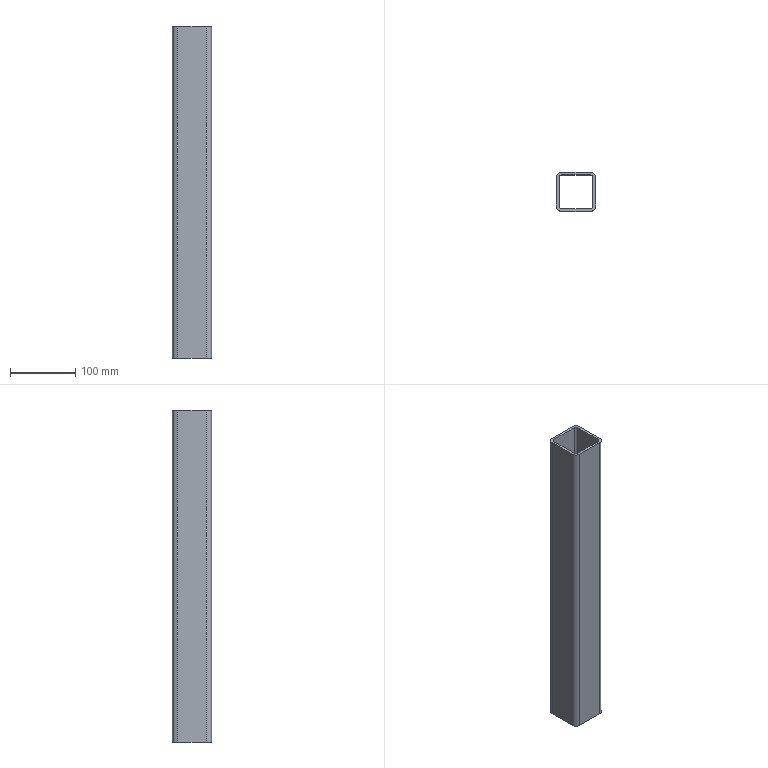Part | SolidWorks | features ICE 1, LibraryFeature 1 | 1 solid | 18 faces | box 60 x 60 x 510 mm | volume 435946 mm3 | plane 10 | cylinder 8 | commonest cylinder face diameters 8 x4 16 x4
STEP:
#1=CARTESIAN_POINT('',(22.,30.,0.));
#2=VERTEX_POINT('',#1);
#3=CARTESIAN_POINT('',(-22.,30.,0.));
#4=VERTEX_POINT('',#3);
#5=CARTESIAN_POINT('',(0.,30.,0.));
#6=DIRECTION('',(-1.,0.,0.));
#7=VECTOR('',#6,1000.);
#8=LINE('',#5,#7);
#9=EDGE_CURVE('',#2,#4,#8,.T.);
#10=ORIENTED_EDGE('',*,*,#9,.T.);
#11=CARTESIAN_POINT('',(-22.,30.,510.));
#12=VERTEX_POINT('',#11);
#13=CARTESIAN_POINT('',(-22.,30.,510.));
#14=DIRECTION('',(0.,0.,-1.));
#15=VECTOR('',#14,1000.);
#16=LINE('',#13,#15);
#17=EDGE_CURVE('',#12,#4,#16,.T.);
#18=ORIENTED_EDGE('',*,*,#17,.F.);
#19=CARTESIAN_POINT('',(22.,30.,510.));
#20=VERTEX_POINT('',#19);
#21=CARTESIAN_POINT('',(0.,30.,510.));
#22=DIRECTION('',(-1.,0.,0.));
#23=VECTOR('',#22,1000.);
#24=LINE('',#21,#23);
#25=EDGE_CURVE('',#20,#12,#24,.T.);
#26=ORIENTED_EDGE('',*,*,#25,.F.);
#27=CARTESIAN_POINT('',(22.,30.,510.));
#28=DIRECTION('',(0.,0.,-1.));
#29=VECTOR('',#28,1000.);
#30=LINE('',#27,#29);
#31=EDGE_CURVE('',#20,#2,#30,.T.);
#32=ORIENTED_EDGE('',*,*,#31,.T.);
#33=EDGE_LOOP('',(#10,#18,#26,#32));
#34=FACE_OUTER_BOUND('',#33,.T.);
#35=CARTESIAN_POINT('',(0.,30.,510.));
#36=DIRECTION('',(0.,-1.,0.));
#37=DIRECTION('',(0.,0.,-1.));
#38=AXIS2_PLACEMENT_3D('',#35,#36,#37);
#39=PLANE('',#38);
#40=ADVANCED_FACE('',(#34),#39,.F.);
#41=CARTESIAN_POINT('',(-30.,22.,0.));
#42=VERTEX_POINT('',#41);
#43=CARTESIAN_POINT('',(-22.,22.,0.));
#44=DIRECTION('',(0.,0.,1.));
#45=DIRECTION('',(1.,0.,0.));
#46=AXIS2_PLACEMENT_3D('',#43,#44,#45);
#47=CIRCLE('',#46,8.);
#48=EDGE_CURVE('',#4,#42,#47,.T.);
#49=ORIENTED_EDGE('',*,*,#48,.T.);
#50=CARTESIAN_POINT('',(-30.,22.,510.));
#51=VERTEX_POINT('',#50);
#52=CARTESIAN_POINT('',(-30.,22.,510.));
#53=DIRECTION('',(0.,0.,-1.));
#54=VECTOR('',#53,1000.);
#55=LINE('',#52,#54);
#56=EDGE_CURVE('',#51,#42,#55,.T.);
#57=ORIENTED_EDGE('',*,*,#56,.F.);
#58=CARTESIAN_POINT('',(-22.,22.,510.));
#59=DIRECTION('',(0.,0.,1.));
#60=DIRECTION('',(1.,0.,0.));
#61=AXIS2_PLACEMENT_3D('',#58,#59,#60);
#62=CIRCLE('',#61,8.);
#63=EDGE_CURVE('',#12,#51,#62,.T.);
#64=ORIENTED_EDGE('',*,*,#63,.F.);
#65=ORIENTED_EDGE('',*,*,#17,.T.);
#66=EDGE_LOOP('',(#49,#57,#64,#65));
#67=FACE_OUTER_BOUND('',#66,.T.);
#68=CARTESIAN_POINT('',(-22.,22.,510.));
#69=DIRECTION('',(0.,0.,-1.));
#70=DIRECTION('',(-1.,0.,0.));
#71=AXIS2_PLACEMENT_3D('',#68,#69,#70);
#72=CYLINDRICAL_SURFACE('',#71,8.);
#73=ADVANCED_FACE('',(#67),#72,.T.);
#74=CARTESIAN_POINT('',(-30.,-22.,0.));
#75=VERTEX_POINT('',#74);
#76=CARTESIAN_POINT('',(-30.,0.,0.));
#77=DIRECTION('',(0.,1.,0.));
#78=VECTOR('',#77,1000.);
#79=LINE('',#76,#78);
#80=EDGE_CURVE('',#75,#42,#79,.T.);
#81=ORIENTED_EDGE('',*,*,#80,.F.);
#82=CARTESIAN_POINT('',(-30.,-22.,510.));
#83=VERTEX_POINT('',#82);
#84=CARTESIAN_POINT('',(-30.,-22.,510.));
#85=DIRECTION('',(0.,0.,-1.));
#86=VECTOR('',#85,1000.);
#87=LINE('',#84,#86);
#88=EDGE_CURVE('',#83,#75,#87,.T.);
#89=ORIENTED_EDGE('',*,*,#88,.F.);
#90=CARTESIAN_POINT('',(-30.,0.,510.));
#91=DIRECTION('',(0.,1.,0.));
#92=VECTOR('',#91,1000.);
#93=LINE('',#90,#92);
#94=EDGE_CURVE('',#83,#51,#93,.T.);
#95=ORIENTED_EDGE('',*,*,#94,.T.);
#96=ORIENTED_EDGE('',*,*,#56,.T.);
#97=EDGE_LOOP('',(#81,#89,#95,#96));
#98=FACE_OUTER_BOUND('',#97,.T.);
#99=CARTESIAN_POINT('',(-30.,0.,510.));
#100=DIRECTION('',(-1.,0.,0.));
#101=DIRECTION('',(0.,0.,1.));
#102=AXIS2_PLACEMENT_3D('',#99,#100,#101);
#103=PLANE('',#102);
#104=ADVANCED_FACE('',(#98),#103,.T.);
#105=CARTESIAN_POINT('',(-22.,-30.,0.));
#106=VERTEX_POINT('',#105);
#107=CARTESIAN_POINT('',(-22.,-22.,0.));
#108=DIRECTION('',(0.,0.,1.));
#109=DIRECTION('',(1.,0.,0.));
#110=AXIS2_PLACEMENT_3D('',#107,#108,#109);
#111=CIRCLE('',#110,8.);
#112=EDGE_CURVE('',#75,#106,#111,.T.);
#113=ORIENTED_EDGE('',*,*,#112,.T.);
#114=CARTESIAN_POINT('',(-22.,-30.,510.));
#115=VERTEX_POINT('',#114);
#116=CARTESIAN_POINT('',(-22.,-30.,510.));
#117=DIRECTION('',(0.,0.,-1.));
#118=VECTOR('',#117,1000.);
#119=LINE('',#116,#118);
#120=EDGE_CURVE('',#115,#106,#119,.T.);
#121=ORIENTED_EDGE('',*,*,#120,.F.);
#122=CARTESIAN_POINT('',(-22.,-22.,510.));
#123=DIRECTION('',(0.,0.,1.));
#124=DIRECTION('',(1.,0.,0.));
#125=AXIS2_PLACEMENT_3D('',#122,#123,#124);
#126=CIRCLE('',#125,8.);
#127=EDGE_CURVE('',#83,#115,#126,.T.);
#128=ORIENTED_EDGE('',*,*,#127,.F.);
#129=ORIENTED_EDGE('',*,*,#88,.T.);
#130=EDGE_LOOP('',(#113,#121,#128,#129));
#131=FACE_OUTER_BOUND('',#130,.T.);
#132=CARTESIAN_POINT('',(-22.,-22.,510.));
#133=DIRECTION('',(0.,0.,-1.));
#134=DIRECTION('',(-1.,0.,0.));
#135=AXIS2_PLACEMENT_3D('',#132,#133,#134);
#136=CYLINDRICAL_SURFACE('',#135,8.);
#137=ADVANCED_FACE('',(#131),#136,.T.);
#138=CARTESIAN_POINT('',(22.,-30.,0.));
#139=VERTEX_POINT('',#138);
#140=CARTESIAN_POINT('',(0.,-30.,0.));
#141=DIRECTION('',(1.,0.,0.));
#142=VECTOR('',#141,1000.);
#143=LINE('',#140,#142);
#144=EDGE_CURVE('',#106,#139,#143,.T.);
#145=ORIENTED_EDGE('',*,*,#144,.T.);
#146=CARTESIAN_POINT('',(22.,-30.,510.));
#147=VERTEX_POINT('',#146);
#148=CARTESIAN_POINT('',(22.,-30.,510.));
#149=DIRECTION('',(0.,0.,-1.));
#150=VECTOR('',#149,1000.);
#151=LINE('',#148,#150);
#152=EDGE_CURVE('',#147,#139,#151,.T.);
#153=ORIENTED_EDGE('',*,*,#152,.F.);
#154=CARTESIAN_POINT('',(0.,-30.,510.));
#155=DIRECTION('',(1.,0.,0.));
#156=VECTOR('',#155,1000.);
#157=LINE('',#154,#156);
#158=EDGE_CURVE('',#115,#147,#157,.T.);
#159=ORIENTED_EDGE('',*,*,#158,.F.);
#160=ORIENTED_EDGE('',*,*,#120,.T.);
#161=EDGE_LOOP('',(#145,#153,#159,#160));
#162=FACE_OUTER_BOUND('',#161,.T.);
#163=CARTESIAN_POINT('',(0.,-30.,510.));
#164=DIRECTION('',(0.,1.,0.));
#165=DIRECTION('',(0.,0.,1.));
#166=AXIS2_PLACEMENT_3D('',#163,#164,#165);
#167=PLANE('',#166);
#168=ADVANCED_FACE('',(#162),#167,.F.);
#169=CARTESIAN_POINT('',(30.,-22.,0.));
#170=VERTEX_POINT('',#169);
#171=CARTESIAN_POINT('',(22.,-22.,0.));
#172=DIRECTION('',(0.,0.,1.));
#173=DIRECTION('',(1.,0.,0.));
#174=AXIS2_PLACEMENT_3D('',#171,#172,#173);
#175=CIRCLE('',#174,8.);
#176=EDGE_CURVE('',#139,#170,#175,.T.);
#177=ORIENTED_EDGE('',*,*,#176,.T.);
#178=CARTESIAN_POINT('',(30.,-22.,510.));
#179=VERTEX_POINT('',#178);
#180=CARTESIAN_POINT('',(30.,-22.,510.));
#181=DIRECTION('',(0.,0.,-1.));
#182=VECTOR('',#181,1000.);
#183=LINE('',#180,#182);
#184=EDGE_CURVE('',#179,#170,#183,.T.);
#185=ORIENTED_EDGE('',*,*,#184,.F.);
#186=CARTESIAN_POINT('',(22.,-22.,510.));
#187=DIRECTION('',(0.,0.,1.));
#188=DIRECTION('',(1.,0.,0.));
#189=AXIS2_PLACEMENT_3D('',#186,#187,#188);
#190=CIRCLE('',#189,8.);
#191=EDGE_CURVE('',#147,#179,#190,.T.);
#192=ORIENTED_EDGE('',*,*,#191,.F.);
#193=ORIENTED_EDGE('',*,*,#152,.T.);
#194=EDGE_LOOP('',(#177,#185,#192,#193));
#195=FACE_OUTER_BOUND('',#194,.T.);
#196=CARTESIAN_POINT('',(22.,-22.,510.));
#197=DIRECTION('',(0.,0.,-1.));
#198=DIRECTION('',(-1.,0.,0.));
#199=AXIS2_PLACEMENT_3D('',#196,#197,#198);
#200=CYLINDRICAL_SURFACE('',#199,8.);
#201=ADVANCED_FACE('',(#195),#200,.T.);
#202=CARTESIAN_POINT('',(30.,22.,0.));
#203=VERTEX_POINT('',#202);
#204=CARTESIAN_POINT('',(30.,0.,0.));
#205=DIRECTION('',(0.,-1.,0.));
#206=VECTOR('',#205,1000.);
#207=LINE('',#204,#206);
#208=EDGE_CURVE('',#203,#170,#207,.T.);
#209=ORIENTED_EDGE('',*,*,#208,.F.);
#210=CARTESIAN_POINT('',(30.,22.,510.));
#211=VERTEX_POINT('',#210);
#212=CARTESIAN_POINT('',(30.,22.,510.));
#213=DIRECTION('',(0.,0.,-1.));
#214=VECTOR('',#213,1000.);
#215=LINE('',#212,#214);
#216=EDGE_CURVE('',#211,#203,#215,.T.);
#217=ORIENTED_EDGE('',*,*,#216,.F.);
#218=CARTESIAN_POINT('',(30.,0.,510.));
#219=DIRECTION('',(0.,-1.,0.));
#220=VECTOR('',#219,1000.);
#221=LINE('',#218,#220);
#222=EDGE_CURVE('',#211,#179,#221,.T.);
#223=ORIENTED_EDGE('',*,*,#222,.T.);
#224=ORIENTED_EDGE('',*,*,#184,.T.);
#225=EDGE_LOOP('',(#209,#217,#223,#224));
#226=FACE_OUTER_BOUND('',#225,.T.);
#227=CARTESIAN_POINT('',(30.,0.,510.));
#228=DIRECTION('',(1.,0.,0.));
#229=DIRECTION('',(0.,0.,-1.));
#230=AXIS2_PLACEMENT_3D('',#227,#228,#229);
#231=PLANE('',#230);
#232=ADVANCED_FACE('',(#226),#231,.T.);
#233=CARTESIAN_POINT('',(-26.,-22.,0.));
#234=VERTEX_POINT('',#233);
#235=CARTESIAN_POINT('',(-22.,-26.,0.));
#236=VERTEX_POINT('',#235);
#237=CARTESIAN_POINT('',(-22.,-22.,0.));
#238=DIRECTION('',(0.,0.,1.));
#239=DIRECTION('',(1.,0.,0.));
#240=AXIS2_PLACEMENT_3D('',#237,#238,#239);
#241=CIRCLE('',#240,4.);
#242=EDGE_CURVE('',#234,#236,#241,.T.);
#243=ORIENTED_EDGE('',*,*,#242,.F.);
#244=CARTESIAN_POINT('',(-26.,-22.,510.));
#245=VERTEX_POINT('',#244);
#246=CARTESIAN_POINT('',(-26.,-22.,510.));
#247=DIRECTION('',(0.,0.,-1.));
#248=VECTOR('',#247,1000.);
#249=LINE('',#246,#248);
#250=EDGE_CURVE('',#245,#234,#249,.T.);
#251=ORIENTED_EDGE('',*,*,#250,.F.);
#252=CARTESIAN_POINT('',(-22.,-26.,510.));
#253=VERTEX_POINT('',#252);
#254=CARTESIAN_POINT('',(-22.,-22.,510.));
#255=DIRECTION('',(0.,0.,1.));
#256=DIRECTION('',(1.,0.,0.));
#257=AXIS2_PLACEMENT_3D('',#254,#255,#256);
#258=CIRCLE('',#257,4.);
#259=EDGE_CURVE('',#245,#253,#258,.T.);
#260=ORIENTED_EDGE('',*,*,#259,.T.);
#261=CARTESIAN_POINT('',(-22.,-26.,510.));
#262=DIRECTION('',(0.,0.,-1.));
#263=VECTOR('',#262,1000.);
#264=LINE('',#261,#263);
#265=EDGE_CURVE('',#253,#236,#264,.T.);
#266=ORIENTED_EDGE('',*,*,#265,.T.);
#267=EDGE_LOOP('',(#243,#251,#260,#266));
#268=FACE_OUTER_BOUND('',#267,.T.);
#269=CARTESIAN_POINT('',(-22.,-22.,510.));
#270=DIRECTION('',(0.,0.,-1.));
#271=DIRECTION('',(-1.,0.,0.));
#272=AXIS2_PLACEMENT_3D('',#269,#270,#271);
#273=CYLINDRICAL_SURFACE('',#272,4.);
#274=ADVANCED_FACE('',(#268),#273,.F.);
#275=CARTESIAN_POINT('',(-26.,22.,0.));
#276=VERTEX_POINT('',#275);
#277=CARTESIAN_POINT('',(-26.,0.,0.));
#278=DIRECTION('',(0.,1.,0.));
#279=VECTOR('',#278,1000.);
#280=LINE('',#277,#279);
#281=EDGE_CURVE('',#234,#276,#280,.T.);
#282=ORIENTED_EDGE('',*,*,#281,.T.);
#283=CARTESIAN_POINT('',(-26.,22.,510.));
#284=VERTEX_POINT('',#283);
#285=CARTESIAN_POINT('',(-26.,22.,510.));
#286=DIRECTION('',(0.,0.,-1.));
#287=VECTOR('',#286,1000.);
#288=LINE('',#285,#287);
#289=EDGE_CURVE('',#284,#276,#288,.T.);
#290=ORIENTED_EDGE('',*,*,#289,.F.);
#291=CARTESIAN_POINT('',(-26.,0.,510.));
#292=DIRECTION('',(0.,1.,0.));
#293=VECTOR('',#292,1000.);
#294=LINE('',#291,#293);
#295=EDGE_CURVE('',#245,#284,#294,.T.);
#296=ORIENTED_EDGE('',*,*,#295,.F.);
#297=ORIENTED_EDGE('',*,*,#250,.T.);
#298=EDGE_LOOP('',(#282,#290,#296,#297));
#299=FACE_OUTER_BOUND('',#298,.T.);
#300=CARTESIAN_POINT('',(-26.,0.,510.));
#301=DIRECTION('',(-1.,0.,0.));
#302=DIRECTION('',(0.,0.,1.));
#303=AXIS2_PLACEMENT_3D('',#300,#301,#302);
#304=PLANE('',#303);
#305=ADVANCED_FACE('',(#299),#304,.F.);
#306=CARTESIAN_POINT('',(-22.,26.,0.));
#307=VERTEX_POINT('',#306);
#308=CARTESIAN_POINT('',(-22.,22.,0.));
#309=DIRECTION('',(0.,0.,1.));
#310=DIRECTION('',(1.,0.,0.));
#311=AXIS2_PLACEMENT_3D('',#308,#309,#310);
#312=CIRCLE('',#311,4.);
#313=EDGE_CURVE('',#307,#276,#312,.T.);
#314=ORIENTED_EDGE('',*,*,#313,.F.);
#315=CARTESIAN_POINT('',(-22.,26.,510.));
#316=VERTEX_POINT('',#315);
#317=CARTESIAN_POINT('',(-22.,26.,510.));
#318=DIRECTION('',(0.,0.,-1.));
#319=VECTOR('',#318,1000.);
#320=LINE('',#317,#319);
#321=EDGE_CURVE('',#316,#307,#320,.T.);
#322=ORIENTED_EDGE('',*,*,#321,.F.);
#323=CARTESIAN_POINT('',(-22.,22.,510.));
#324=DIRECTION('',(0.,0.,1.));
#325=DIRECTION('',(1.,0.,0.));
#326=AXIS2_PLACEMENT_3D('',#323,#324,#325);
#327=CIRCLE('',#326,4.);
#328=EDGE_CURVE('',#316,#284,#327,.T.);
#329=ORIENTED_EDGE('',*,*,#328,.T.);
#330=ORIENTED_EDGE('',*,*,#289,.T.);
#331=EDGE_LOOP('',(#314,#322,#329,#330));
#332=FACE_OUTER_BOUND('',#331,.T.);
#333=CARTESIAN_POINT('',(-22.,22.,510.));
#334=DIRECTION('',(0.,0.,-1.));
#335=DIRECTION('',(-1.,0.,0.));
#336=AXIS2_PLACEMENT_3D('',#333,#334,#335);
#337=CYLINDRICAL_SURFACE('',#336,4.);
#338=ADVANCED_FACE('',(#332),#337,.F.);
#339=CARTESIAN_POINT('',(22.,26.,0.));
#340=VERTEX_POINT('',#339);
#341=CARTESIAN_POINT('',(0.,26.,0.));
#342=DIRECTION('',(-1.,0.,0.));
#343=VECTOR('',#342,1000.);
#344=LINE('',#341,#343);
#345=EDGE_CURVE('',#340,#307,#344,.T.);
#346=ORIENTED_EDGE('',*,*,#345,.F.);
#347=CARTESIAN_POINT('',(22.,26.,510.));
#348=VERTEX_POINT('',#347);
#349=CARTESIAN_POINT('',(22.,26.,510.));
#350=DIRECTION('',(0.,0.,-1.));
#351=VECTOR('',#350,1000.);
#352=LINE('',#349,#351);
#353=EDGE_CURVE('',#348,#340,#352,.T.);
#354=ORIENTED_EDGE('',*,*,#353,.F.);
#355=CARTESIAN_POINT('',(0.,26.,510.));
#356=DIRECTION('',(-1.,0.,0.));
#357=VECTOR('',#356,1000.);
#358=LINE('',#355,#357);
#359=EDGE_CURVE('',#348,#316,#358,.T.);
#360=ORIENTED_EDGE('',*,*,#359,.T.);
#361=ORIENTED_EDGE('',*,*,#321,.T.);
#362=EDGE_LOOP('',(#346,#354,#360,#361));
#363=FACE_OUTER_BOUND('',#362,.T.);
#364=CARTESIAN_POINT('',(0.,26.,510.));
#365=DIRECTION('',(0.,-1.,0.));
#366=DIRECTION('',(0.,0.,-1.));
#367=AXIS2_PLACEMENT_3D('',#364,#365,#366);
#368=PLANE('',#367);
#369=ADVANCED_FACE('',(#363),#368,.T.);
#370=CARTESIAN_POINT('',(26.,22.,0.));
#371=VERTEX_POINT('',#370);
#372=CARTESIAN_POINT('',(22.,22.,0.));
#373=DIRECTION('',(0.,0.,1.));
#374=DIRECTION('',(1.,0.,0.));
#375=AXIS2_PLACEMENT_3D('',#372,#373,#374);
#376=CIRCLE('',#375,4.);
#377=EDGE_CURVE('',#371,#340,#376,.T.);
#378=ORIENTED_EDGE('',*,*,#377,.F.);
#379=CARTESIAN_POINT('',(26.,22.,510.));
#380=VERTEX_POINT('',#379);
#381=CARTESIAN_POINT('',(26.,22.,510.));
#382=DIRECTION('',(0.,0.,-1.));
#383=VECTOR('',#382,1000.);
#384=LINE('',#381,#383);
#385=EDGE_CURVE('',#380,#371,#384,.T.);
#386=ORIENTED_EDGE('',*,*,#385,.F.);
#387=CARTESIAN_POINT('',(22.,22.,510.));
#388=DIRECTION('',(0.,0.,1.));
#389=DIRECTION('',(1.,0.,0.));
#390=AXIS2_PLACEMENT_3D('',#387,#388,#389);
#391=CIRCLE('',#390,4.);
#392=EDGE_CURVE('',#380,#348,#391,.T.);
#393=ORIENTED_EDGE('',*,*,#392,.T.);
#394=ORIENTED_EDGE('',*,*,#353,.T.);
#395=EDGE_LOOP('',(#378,#386,#393,#394));
#396=FACE_OUTER_BOUND('',#395,.T.);
#397=CARTESIAN_POINT('',(22.,22.,510.));
#398=DIRECTION('',(0.,0.,-1.));
#399=DIRECTION('',(-1.,0.,0.));
#400=AXIS2_PLACEMENT_3D('',#397,#398,#399);
#401=CYLINDRICAL_SURFACE('',#400,4.);
#402=ADVANCED_FACE('',(#396),#401,.F.);
#403=CARTESIAN_POINT('',(26.,-22.,0.));
#404=VERTEX_POINT('',#403);
#405=CARTESIAN_POINT('',(26.,0.,0.));
#406=DIRECTION('',(0.,-1.,0.));
#407=VECTOR('',#406,1000.);
#408=LINE('',#405,#407);
#409=EDGE_CURVE('',#371,#404,#408,.T.);
#410=ORIENTED_EDGE('',*,*,#409,.T.);
#411=CARTESIAN_POINT('',(26.,-22.,510.));
#412=VERTEX_POINT('',#411);
#413=CARTESIAN_POINT('',(26.,-22.,510.));
#414=DIRECTION('',(0.,0.,-1.));
#415=VECTOR('',#414,1000.);
#416=LINE('',#413,#415);
#417=EDGE_CURVE('',#412,#404,#416,.T.);
#418=ORIENTED_EDGE('',*,*,#417,.F.);
#419=CARTESIAN_POINT('',(26.,0.,510.));
#420=DIRECTION('',(0.,-1.,0.));
#421=VECTOR('',#420,1000.);
#422=LINE('',#419,#421);
#423=EDGE_CURVE('',#380,#412,#422,.T.);
#424=ORIENTED_EDGE('',*,*,#423,.F.);
#425=ORIENTED_EDGE('',*,*,#385,.T.);
#426=EDGE_LOOP('',(#410,#418,#424,#425));
#427=FACE_OUTER_BOUND('',#426,.T.);
#428=CARTESIAN_POINT('',(26.,0.,510.));
#429=DIRECTION('',(1.,0.,0.));
#430=DIRECTION('',(0.,0.,-1.));
#431=AXIS2_PLACEMENT_3D('',#428,#429,#430);
#432=PLANE('',#431);
#433=ADVANCED_FACE('',(#427),#432,.F.);
#434=CARTESIAN_POINT('',(22.,-26.,0.));
#435=VERTEX_POINT('',#434);
#436=CARTESIAN_POINT('',(22.,-22.,0.));
#437=DIRECTION('',(0.,0.,1.));
#438=DIRECTION('',(1.,0.,0.));
#439=AXIS2_PLACEMENT_3D('',#436,#437,#438);
#440=CIRCLE('',#439,4.);
#441=EDGE_CURVE('',#435,#404,#440,.T.);
#442=ORIENTED_EDGE('',*,*,#441,.F.);
#443=CARTESIAN_POINT('',(22.,-26.,510.));
#444=VERTEX_POINT('',#443);
#445=CARTESIAN_POINT('',(22.,-26.,510.));
#446=DIRECTION('',(0.,0.,-1.));
#447=VECTOR('',#446,1000.);
#448=LINE('',#445,#447);
#449=EDGE_CURVE('',#444,#435,#448,.T.);
#450=ORIENTED_EDGE('',*,*,#449,.F.);
#451=CARTESIAN_POINT('',(22.,-22.,510.));
#452=DIRECTION('',(0.,0.,1.));
#453=DIRECTION('',(1.,0.,0.));
#454=AXIS2_PLACEMENT_3D('',#451,#452,#453);
#455=CIRCLE('',#454,4.);
#456=EDGE_CURVE('',#444,#412,#455,.T.);
#457=ORIENTED_EDGE('',*,*,#456,.T.);
#458=ORIENTED_EDGE('',*,*,#417,.T.);
#459=EDGE_LOOP('',(#442,#450,#457,#458));
#460=FACE_OUTER_BOUND('',#459,.T.);
#461=CARTESIAN_POINT('',(22.,-22.,510.));
#462=DIRECTION('',(0.,0.,-1.));
#463=DIRECTION('',(-1.,0.,0.));
#464=AXIS2_PLACEMENT_3D('',#461,#462,#463);
#465=CYLINDRICAL_SURFACE('',#464,4.);
#466=ADVANCED_FACE('',(#460),#465,.F.);
#467=CARTESIAN_POINT('',(0.,-26.,0.));
#468=DIRECTION('',(1.,0.,0.));
#469=VECTOR('',#468,1000.);
#470=LINE('',#467,#469);
#471=EDGE_CURVE('',#236,#435,#470,.T.);
#472=ORIENTED_EDGE('',*,*,#471,.F.);
#473=ORIENTED_EDGE('',*,*,#265,.F.);
#474=CARTESIAN_POINT('',(0.,-26.,510.));
#475=DIRECTION('',(1.,0.,0.));
#476=VECTOR('',#475,1000.);
#477=LINE('',#474,#476);
#478=EDGE_CURVE('',#253,#444,#477,.T.);
#479=ORIENTED_EDGE('',*,*,#478,.T.);
#480=ORIENTED_EDGE('',*,*,#449,.T.);
#481=EDGE_LOOP('',(#472,#473,#479,#480));
#482=FACE_OUTER_BOUND('',#481,.T.);
#483=CARTESIAN_POINT('',(0.,-26.,510.));
#484=DIRECTION('',(0.,1.,0.));
#485=DIRECTION('',(0.,0.,1.));
#486=AXIS2_PLACEMENT_3D('',#483,#484,#485);
#487=PLANE('',#486);
#488=ADVANCED_FACE('',(#482),#487,.T.);
#489=CARTESIAN_POINT('',(22.,22.,0.));
#490=DIRECTION('',(0.,0.,1.));
#491=DIRECTION('',(1.,0.,0.));
#492=AXIS2_PLACEMENT_3D('',#489,#490,#491);
#493=CIRCLE('',#492,8.);
#494=EDGE_CURVE('',#203,#2,#493,.T.);
#495=ORIENTED_EDGE('',*,*,#494,.T.);
#496=ORIENTED_EDGE('',*,*,#31,.F.);
#497=CARTESIAN_POINT('',(22.,22.,510.));
#498=DIRECTION('',(0.,0.,1.));
#499=DIRECTION('',(1.,0.,0.));
#500=AXIS2_PLACEMENT_3D('',#497,#498,#499);
#501=CIRCLE('',#500,8.);
#502=EDGE_CURVE('',#211,#20,#501,.T.);
#503=ORIENTED_EDGE('',*,*,#502,.F.);
#504=ORIENTED_EDGE('',*,*,#216,.T.);
#505=EDGE_LOOP('',(#495,#496,#503,#504));
#506=FACE_OUTER_BOUND('',#505,.T.);
#507=CARTESIAN_POINT('',(22.,22.,510.));
#508=DIRECTION('',(0.,0.,-1.));
#509=DIRECTION('',(-1.,0.,0.));
#510=AXIS2_PLACEMENT_3D('',#507,#508,#509);
#511=CYLINDRICAL_SURFACE('',#510,8.);
#512=ADVANCED_FACE('',(#506),#511,.T.);
#513=ORIENTED_EDGE('',*,*,#259,.F.);
#514=ORIENTED_EDGE('',*,*,#295,.T.);
#515=ORIENTED_EDGE('',*,*,#328,.F.);
#516=ORIENTED_EDGE('',*,*,#359,.F.);
#517=ORIENTED_EDGE('',*,*,#392,.F.);
#518=ORIENTED_EDGE('',*,*,#423,.T.);
#519=ORIENTED_EDGE('',*,*,#456,.F.);
#520=ORIENTED_EDGE('',*,*,#478,.F.);
#521=EDGE_LOOP('',(#513,#514,#515,#516,#517,#518,#519,#520));
#522=FACE_BOUND('',#521,.T.);
#523=ORIENTED_EDGE('',*,*,#25,.T.);
#524=ORIENTED_EDGE('',*,*,#63,.T.);
#525=ORIENTED_EDGE('',*,*,#94,.F.);
#526=ORIENTED_EDGE('',*,*,#127,.T.);
#527=ORIENTED_EDGE('',*,*,#158,.T.);
#528=ORIENTED_EDGE('',*,*,#191,.T.);
#529=ORIENTED_EDGE('',*,*,#222,.F.);
#530=ORIENTED_EDGE('',*,*,#502,.T.);
#531=EDGE_LOOP('',(#523,#524,#525,#526,#527,#528,#529,#530));
#532=FACE_OUTER_BOUND('',#531,.T.);
#533=CARTESIAN_POINT('',(0.,0.,510.));
#534=DIRECTION('',(0.,0.,1.));
#535=DIRECTION('',(1.,0.,0.));
#536=AXIS2_PLACEMENT_3D('',#533,#534,#535);
#537=PLANE('',#536);
#538=ADVANCED_FACE('',(#522,#532),#537,.T.);
#539=ORIENTED_EDGE('',*,*,#242,.T.);
#540=ORIENTED_EDGE('',*,*,#471,.T.);
#541=ORIENTED_EDGE('',*,*,#441,.T.);
#542=ORIENTED_EDGE('',*,*,#409,.F.);
#543=ORIENTED_EDGE('',*,*,#377,.T.);
#544=ORIENTED_EDGE('',*,*,#345,.T.);
#545=ORIENTED_EDGE('',*,*,#313,.T.);
#546=ORIENTED_EDGE('',*,*,#281,.F.);
#547=EDGE_LOOP('',(#539,#540,#541,#542,#543,#544,#545,#546));
#548=FACE_BOUND('',#547,.T.);
#549=ORIENTED_EDGE('',*,*,#9,.F.);
#550=ORIENTED_EDGE('',*,*,#494,.F.);
#551=ORIENTED_EDGE('',*,*,#208,.T.);
#552=ORIENTED_EDGE('',*,*,#176,.F.);
#553=ORIENTED_EDGE('',*,*,#144,.F.);
#554=ORIENTED_EDGE('',*,*,#112,.F.);
#555=ORIENTED_EDGE('',*,*,#80,.T.);
#556=ORIENTED_EDGE('',*,*,#48,.F.);
#557=EDGE_LOOP('',(#549,#550,#551,#552,#553,#554,#555,#556));
#558=FACE_OUTER_BOUND('',#557,.T.);
#559=CARTESIAN_POINT('',(0.,0.,0.));
#560=DIRECTION('',(0.,0.,1.));
#561=DIRECTION('',(1.,0.,0.));
#562=AXIS2_PLACEMENT_3D('',#559,#560,#561);
#563=PLANE('',#562);
#564=ADVANCED_FACE('',(#548,#558),#563,.F.);
#565=CLOSED_SHELL('',(#40,#73,#104,#137,#168,#201,#232,#274,#305,#338,#369,#402,#433,#466,#488,#512,#538,#564));
#566=MANIFOLD_SOLID_BREP('',#565);
#567=CARTESIAN_POINT('',(0.,0.,0.));
#568=DIRECTION('',(0.,0.,1.));
#569=DIRECTION('',(1.,0.,0.));
#570=AXIS2_PLACEMENT_3D('',#567,#568,#569);
#571=(LENGTH_UNIT()NAMED_UNIT(*)SI_UNIT(.MILLI.,.METRE.));
#572=UNCERTAINTY_MEASURE_WITH_UNIT(LENGTH_MEASURE(0.00001),#571,'','');
#573=(NAMED_UNIT(*)PLANE_ANGLE_UNIT()SI_UNIT($,.RADIAN.));
#574=(NAMED_UNIT(*)SI_UNIT($,.STERADIAN.)SOLID_ANGLE_UNIT());
#575=(GEOMETRIC_REPRESENTATION_CONTEXT(3)GLOBAL_UNCERTAINTY_ASSIGNED_CONTEXT((#572))GLOBAL_UNIT_ASSIGNED_CONTEXT((#571,#573,#574))REPRESENTATION_CONTEXT('',''));
#576=ADVANCED_BREP_SHAPE_REPRESENTATION('',(#566,#570),#575);